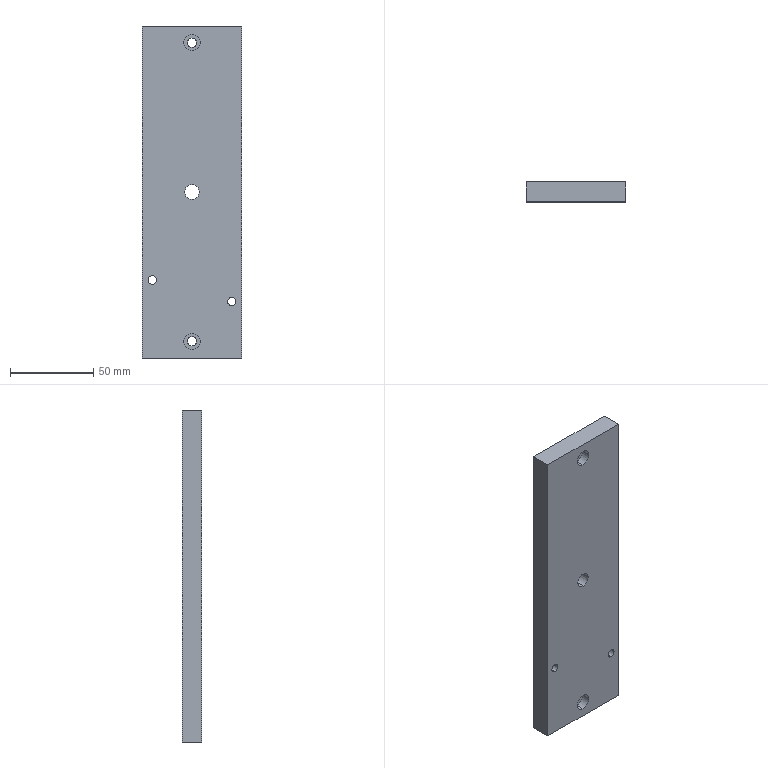Part | STEP file | PN_0018 | 1 solid | 28 faces | box 60 x 12 x 200 mm | volume 140928 mm3 | cylinder 18 | plane 10 | commonest cylinder face diameters 5 x4 5.5 x4 10 x4 16 x4 8.8 x2